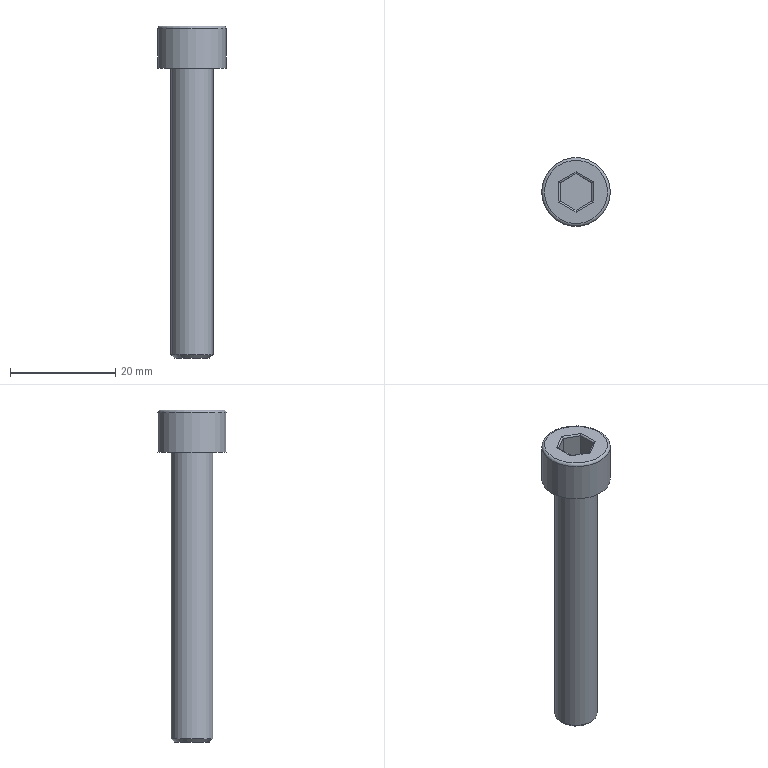Part | STEP file | 200 mesh_id90_xmt | 1 solid | 20 faces | box 13 x 13 x 63 mm | volume 3664 mm3 | plane 10 | cylinder 8 | torus 1 | cone 1 | commonest cylinder face diameters 0.6 x6 8 x1 13 x1
STEP:
#1=CARTESIAN_POINT('',(-16967.884,-4114.08,125.258));
#2=VERTEX_POINT('',#1);
#3=CARTESIAN_POINT('',(-16971.184,-4112.174,125.258));
#4=VERTEX_POINT('',#3);
#5=CARTESIAN_POINT('',(-16969.534,-4113.127,125.258));
#6=DIRECTION('',(-0.866,0.5,0.));
#7=VECTOR('',#6,1.);
#8=LINE('',#5,#7);
#9=EDGE_CURVE('',#2,#4,#8,.T.);
#10=ORIENTED_EDGE('',*,*,#9,.T.);
#11=CARTESIAN_POINT('',(-16971.184,-4108.364,125.258));
#12=VERTEX_POINT('',#11);
#13=CARTESIAN_POINT('',(-16971.184,-4110.269,125.258));
#14=DIRECTION('',(0.,1.,0.));
#15=VECTOR('',#14,1.);
#16=LINE('',#13,#15);
#17=EDGE_CURVE('',#4,#12,#16,.T.);
#18=ORIENTED_EDGE('',*,*,#17,.T.);
#19=CARTESIAN_POINT('',(-16967.884,-4106.459,125.258));
#20=VERTEX_POINT('',#19);
#21=CARTESIAN_POINT('',(-16969.534,-4107.411,125.258));
#22=DIRECTION('',(0.866,0.5,0.));
#23=VECTOR('',#22,1.);
#24=LINE('',#21,#23);
#25=EDGE_CURVE('',#12,#20,#24,.T.);
#26=ORIENTED_EDGE('',*,*,#25,.T.);
#27=CARTESIAN_POINT('',(-16964.584,-4108.364,125.258));
#28=VERTEX_POINT('',#27);
#29=CARTESIAN_POINT('',(-16966.234,-4107.411,125.258));
#30=DIRECTION('',(0.866,-0.5,0.));
#31=VECTOR('',#30,1.);
#32=LINE('',#29,#31);
#33=EDGE_CURVE('',#20,#28,#32,.T.);
#34=ORIENTED_EDGE('',*,*,#33,.T.);
#35=CARTESIAN_POINT('',(-16964.584,-4112.174,125.258));
#36=VERTEX_POINT('',#35);
#37=CARTESIAN_POINT('',(-16964.584,-4110.269,125.258));
#38=DIRECTION('',(0.,-1.,0.));
#39=VECTOR('',#38,1.);
#40=LINE('',#37,#39);
#41=EDGE_CURVE('',#28,#36,#40,.T.);
#42=ORIENTED_EDGE('',*,*,#41,.T.);
#43=CARTESIAN_POINT('',(-16966.234,-4113.127,125.258));
#44=DIRECTION('',(-0.866,-0.5,0.));
#45=VECTOR('',#44,1.);
#46=LINE('',#43,#45);
#47=EDGE_CURVE('',#36,#2,#46,.T.);
#48=ORIENTED_EDGE('',*,*,#47,.T.);
#49=EDGE_LOOP('',(#10,#18,#26,#34,#42,#48));
#50=FACE_BOUND('',#49,.T.);
#51=CARTESIAN_POINT('',(-16961.884,-4110.269,125.258));
#52=VERTEX_POINT('',#51);
#53=CARTESIAN_POINT('',(-16967.884,-4110.269,125.258));
#54=DIRECTION('',(0.,0.,1.));
#55=DIRECTION('',(1.,0.,0.));
#56=AXIS2_PLACEMENT_3D('',#53,#54,#55);
#57=CIRCLE('',#56,6.);
#58=EDGE_CURVE('',#52,#52,#57,.T.);
#59=ORIENTED_EDGE('',*,*,#58,.T.);
#60=EDGE_LOOP('',(#59));
#61=FACE_BOUND('',#60,.T.);
#62=CARTESIAN_POINT('',(-16967.884,-4110.269,125.258));
#63=DIRECTION('',(0.,0.,1.));
#64=DIRECTION('',(1.,0.,0.));
#65=AXIS2_PLACEMENT_3D('',#62,#63,#64);
#66=PLANE('',#65);
#67=ADVANCED_FACE('',(#50,#61),#66,.T.);
#68=CARTESIAN_POINT('',(-16971.884,-4110.269,62.858));
#69=VERTEX_POINT('',#68);
#70=CARTESIAN_POINT('',(-16967.884,-4110.269,62.858));
#71=DIRECTION('',(0.,0.,1.));
#72=DIRECTION('',(-1.,0.,0.));
#73=AXIS2_PLACEMENT_3D('',#70,#71,#72);
#74=CIRCLE('',#73,4.);
#75=EDGE_CURVE('',#69,#69,#74,.T.);
#76=ORIENTED_EDGE('',*,*,#75,.T.);
#77=EDGE_LOOP('',(#76));
#78=FACE_BOUND('',#77,.T.);
#79=CARTESIAN_POINT('',(-16971.884,-4110.269,117.258));
#80=VERTEX_POINT('',#79);
#81=CARTESIAN_POINT('',(-16967.884,-4110.269,117.258));
#82=DIRECTION('',(0.,0.,1.));
#83=DIRECTION('',(-1.,0.,0.));
#84=AXIS2_PLACEMENT_3D('',#81,#82,#83);
#85=CIRCLE('',#84,4.);
#86=EDGE_CURVE('',#80,#80,#85,.T.);
#87=ORIENTED_EDGE('',*,*,#86,.F.);
#88=EDGE_LOOP('',(#87));
#89=FACE_BOUND('',#88,.T.);
#90=CARTESIAN_POINT('',(-16967.884,-4110.269,117.258));
#91=DIRECTION('',(0.,0.,-1.));
#92=DIRECTION('',(1.,0.,0.));
#93=AXIS2_PLACEMENT_3D('',#90,#91,#92);
#94=CYLINDRICAL_SURFACE('',#93,4.);
#95=ADVANCED_FACE('',(#78,#89),#94,.T.);
#96=ORIENTED_EDGE('',*,*,#86,.T.);
#97=EDGE_LOOP('',(#96));
#98=FACE_BOUND('',#97,.T.);
#99=CARTESIAN_POINT('',(-16961.384,-4110.269,117.258));
#100=VERTEX_POINT('',#99);
#101=CARTESIAN_POINT('',(-16967.884,-4110.269,117.258));
#102=DIRECTION('',(0.,0.,1.));
#103=DIRECTION('',(1.,0.,0.));
#104=AXIS2_PLACEMENT_3D('',#101,#102,#103);
#105=CIRCLE('',#104,6.5);
#106=EDGE_CURVE('',#100,#100,#105,.T.);
#107=ORIENTED_EDGE('',*,*,#106,.F.);
#108=EDGE_LOOP('',(#107));
#109=FACE_BOUND('',#108,.T.);
#110=CARTESIAN_POINT('',(-16967.884,-4110.269,117.258));
#111=DIRECTION('',(0.,0.,-1.));
#112=DIRECTION('',(-1.,0.,0.));
#113=AXIS2_PLACEMENT_3D('',#110,#111,#112);
#114=PLANE('',#113);
#115=ADVANCED_FACE('',(#98,#109),#114,.T.);
#116=CARTESIAN_POINT('',(-16961.384,-4110.269,124.758));
#117=VERTEX_POINT('',#116);
#118=CARTESIAN_POINT('',(-16967.884,-4110.269,124.758));
#119=DIRECTION('',(0.,0.,-1.));
#120=DIRECTION('',(1.,0.,0.));
#121=AXIS2_PLACEMENT_3D('',#118,#119,#120);
#122=CIRCLE('',#121,6.5);
#123=EDGE_CURVE('',#117,#117,#122,.T.);
#124=ORIENTED_EDGE('',*,*,#123,.T.);
#125=EDGE_LOOP('',(#124));
#126=FACE_BOUND('',#125,.T.);
#127=ORIENTED_EDGE('',*,*,#106,.T.);
#128=EDGE_LOOP('',(#127));
#129=FACE_BOUND('',#128,.T.);
#130=CARTESIAN_POINT('',(-16967.884,-4110.269,117.258));
#131=DIRECTION('',(0.,0.,1.));
#132=DIRECTION('',(1.,0.,0.));
#133=AXIS2_PLACEMENT_3D('',#130,#131,#132);
#134=CYLINDRICAL_SURFACE('',#133,6.5);
#135=ADVANCED_FACE('',(#126,#129),#134,.T.);
#136=ORIENTED_EDGE('',*,*,#58,.F.);
#137=EDGE_LOOP('',(#136));
#138=FACE_BOUND('',#137,.T.);
#139=ORIENTED_EDGE('',*,*,#123,.F.);
#140=EDGE_LOOP('',(#139));
#141=FACE_BOUND('',#140,.T.);
#142=CARTESIAN_POINT('',(-16967.884,-4110.269,124.758));
#143=DIRECTION('',(0.,0.,1.));
#144=DIRECTION('',(1.,0.,0.));
#145=AXIS2_PLACEMENT_3D('',#142,#143,#144);
#146=TOROIDAL_SURFACE('',#145,6.,0.5);
#147=ADVANCED_FACE('',(#138,#141),#146,.T.);
#148=CARTESIAN_POINT('',(-16970.884,-4112.001,124.958));
#149=VERTEX_POINT('',#148);
#150=CARTESIAN_POINT('',(-16970.884,-4112.001,120.258));
#151=VERTEX_POINT('',#150);
#152=CARTESIAN_POINT('',(-16970.884,-4112.001,120.258));
#153=DIRECTION('',(0.,0.,-1.));
#154=VECTOR('',#153,1.);
#155=LINE('',#152,#154);
#156=EDGE_CURVE('',#149,#151,#155,.T.);
#157=ORIENTED_EDGE('',*,*,#156,.F.);
#158=CARTESIAN_POINT('',(-16967.884,-4113.733,124.958));
#159=VERTEX_POINT('',#158);
#160=CARTESIAN_POINT('',(-16967.884,-4113.733,124.958));
#161=DIRECTION('',(0.866,-0.5,0.));
#162=VECTOR('',#161,1.);
#163=LINE('',#160,#162);
#164=EDGE_CURVE('',#149,#159,#163,.T.);
#165=ORIENTED_EDGE('',*,*,#164,.T.);
#166=CARTESIAN_POINT('',(-16967.884,-4113.733,120.258));
#167=VERTEX_POINT('',#166);
#168=CARTESIAN_POINT('',(-16967.884,-4113.733,120.258));
#169=DIRECTION('',(0.,0.,-1.));
#170=VECTOR('',#169,1.);
#171=LINE('',#168,#170);
#172=EDGE_CURVE('',#159,#167,#171,.T.);
#173=ORIENTED_EDGE('',*,*,#172,.T.);
#174=CARTESIAN_POINT('',(-16967.884,-4113.733,120.258));
#175=DIRECTION('',(0.866,-0.5,0.));
#176=VECTOR('',#175,1.);
#177=LINE('',#174,#176);
#178=EDGE_CURVE('',#151,#167,#177,.T.);
#179=ORIENTED_EDGE('',*,*,#178,.F.);
#180=EDGE_LOOP('',(#157,#165,#173,#179));
#181=FACE_OUTER_BOUND('',#180,.T.);
#182=CARTESIAN_POINT('',(-16967.884,-4113.733,120.258));
#183=DIRECTION('',(0.5,0.866,0.));
#184=DIRECTION('',(-0.866,0.5,0.));
#185=AXIS2_PLACEMENT_3D('',#182,#183,#184);
#186=PLANE('',#185);
#187=ADVANCED_FACE('',(#181),#186,.T.);
#188=CARTESIAN_POINT('',(-16970.884,-4108.537,124.958));
#189=VERTEX_POINT('',#188);
#190=CARTESIAN_POINT('',(-16970.884,-4108.537,120.258));
#191=VERTEX_POINT('',#190);
#192=CARTESIAN_POINT('',(-16970.884,-4108.537,120.258));
#193=DIRECTION('',(0.,0.,-1.));
#194=VECTOR('',#193,1.);
#195=LINE('',#192,#194);
#196=EDGE_CURVE('',#189,#191,#195,.T.);
#197=ORIENTED_EDGE('',*,*,#196,.F.);
#198=CARTESIAN_POINT('',(-16970.884,-4112.001,124.958));
#199=DIRECTION('',(0.,-1.,0.));
#200=VECTOR('',#199,1.);
#201=LINE('',#198,#200);
#202=EDGE_CURVE('',#189,#149,#201,.T.);
#203=ORIENTED_EDGE('',*,*,#202,.T.);
#204=ORIENTED_EDGE('',*,*,#156,.T.);
#205=CARTESIAN_POINT('',(-16970.884,-4112.001,120.258));
#206=DIRECTION('',(0.,-1.,0.));
#207=VECTOR('',#206,1.);
#208=LINE('',#205,#207);
#209=EDGE_CURVE('',#191,#151,#208,.T.);
#210=ORIENTED_EDGE('',*,*,#209,.F.);
#211=EDGE_LOOP('',(#197,#203,#204,#210));
#212=FACE_OUTER_BOUND('',#211,.T.);
#213=CARTESIAN_POINT('',(-16970.884,-4112.001,120.258));
#214=DIRECTION('',(1.,0.,0.));
#215=DIRECTION('',(0.,0.,-1.));
#216=AXIS2_PLACEMENT_3D('',#213,#214,#215);
#217=PLANE('',#216);
#218=ADVANCED_FACE('',(#212),#217,.T.);
#219=CARTESIAN_POINT('',(-16967.884,-4106.805,124.958));
#220=VERTEX_POINT('',#219);
#221=CARTESIAN_POINT('',(-16967.884,-4106.805,120.258));
#222=VERTEX_POINT('',#221);
#223=CARTESIAN_POINT('',(-16967.884,-4106.805,120.258));
#224=DIRECTION('',(0.,0.,-1.));
#225=VECTOR('',#224,1.);
#226=LINE('',#223,#225);
#227=EDGE_CURVE('',#220,#222,#226,.T.);
#228=ORIENTED_EDGE('',*,*,#227,.F.);
#229=CARTESIAN_POINT('',(-16970.884,-4108.537,124.958));
#230=DIRECTION('',(-0.866,-0.5,0.));
#231=VECTOR('',#230,1.);
#232=LINE('',#229,#231);
#233=EDGE_CURVE('',#220,#189,#232,.T.);
#234=ORIENTED_EDGE('',*,*,#233,.T.);
#235=ORIENTED_EDGE('',*,*,#196,.T.);
#236=CARTESIAN_POINT('',(-16970.884,-4108.537,120.258));
#237=DIRECTION('',(-0.866,-0.5,0.));
#238=VECTOR('',#237,1.);
#239=LINE('',#236,#238);
#240=EDGE_CURVE('',#222,#191,#239,.T.);
#241=ORIENTED_EDGE('',*,*,#240,.F.);
#242=EDGE_LOOP('',(#228,#234,#235,#241));
#243=FACE_OUTER_BOUND('',#242,.T.);
#244=CARTESIAN_POINT('',(-16970.884,-4108.537,120.258));
#245=DIRECTION('',(0.5,-0.866,0.));
#246=DIRECTION('',(0.866,0.5,0.));
#247=AXIS2_PLACEMENT_3D('',#244,#245,#246);
#248=PLANE('',#247);
#249=ADVANCED_FACE('',(#243),#248,.T.);
#250=CARTESIAN_POINT('',(-16964.884,-4108.537,124.958));
#251=VERTEX_POINT('',#250);
#252=CARTESIAN_POINT('',(-16964.884,-4108.537,120.258));
#253=VERTEX_POINT('',#252);
#254=CARTESIAN_POINT('',(-16964.884,-4108.537,120.258));
#255=DIRECTION('',(0.,0.,-1.));
#256=VECTOR('',#255,1.);
#257=LINE('',#254,#256);
#258=EDGE_CURVE('',#251,#253,#257,.T.);
#259=ORIENTED_EDGE('',*,*,#258,.F.);
#260=CARTESIAN_POINT('',(-16967.884,-4106.805,124.958));
#261=DIRECTION('',(-0.866,0.5,0.));
#262=VECTOR('',#261,1.);
#263=LINE('',#260,#262);
#264=EDGE_CURVE('',#251,#220,#263,.T.);
#265=ORIENTED_EDGE('',*,*,#264,.T.);
#266=ORIENTED_EDGE('',*,*,#227,.T.);
#267=CARTESIAN_POINT('',(-16967.884,-4106.805,120.258));
#268=DIRECTION('',(-0.866,0.5,0.));
#269=VECTOR('',#268,1.);
#270=LINE('',#267,#269);
#271=EDGE_CURVE('',#253,#222,#270,.T.);
#272=ORIENTED_EDGE('',*,*,#271,.F.);
#273=EDGE_LOOP('',(#259,#265,#266,#272));
#274=FACE_OUTER_BOUND('',#273,.T.);
#275=CARTESIAN_POINT('',(-16967.884,-4106.805,120.258));
#276=DIRECTION('',(-0.5,-0.866,0.));
#277=DIRECTION('',(0.866,-0.5,0.));
#278=AXIS2_PLACEMENT_3D('',#275,#276,#277);
#279=PLANE('',#278);
#280=ADVANCED_FACE('',(#274),#279,.T.);
#281=CARTESIAN_POINT('',(-16964.884,-4112.001,124.958));
#282=VERTEX_POINT('',#281);
#283=CARTESIAN_POINT('',(-16964.884,-4112.001,120.258));
#284=VERTEX_POINT('',#283);
#285=CARTESIAN_POINT('',(-16964.884,-4112.001,120.258));
#286=DIRECTION('',(0.,0.,-1.));
#287=VECTOR('',#286,1.);
#288=LINE('',#285,#287);
#289=EDGE_CURVE('',#282,#284,#288,.T.);
#290=ORIENTED_EDGE('',*,*,#289,.F.);
#291=CARTESIAN_POINT('',(-16964.884,-4108.537,124.958));
#292=DIRECTION('',(0.,1.,0.));
#293=VECTOR('',#292,1.);
#294=LINE('',#291,#293);
#295=EDGE_CURVE('',#282,#251,#294,.T.);
#296=ORIENTED_EDGE('',*,*,#295,.T.);
#297=ORIENTED_EDGE('',*,*,#258,.T.);
#298=CARTESIAN_POINT('',(-16964.884,-4108.537,120.258));
#299=DIRECTION('',(0.,1.,0.));
#300=VECTOR('',#299,1.);
#301=LINE('',#298,#300);
#302=EDGE_CURVE('',#284,#253,#301,.T.);
#303=ORIENTED_EDGE('',*,*,#302,.F.);
#304=EDGE_LOOP('',(#290,#296,#297,#303));
#305=FACE_OUTER_BOUND('',#304,.T.);
#306=CARTESIAN_POINT('',(-16964.884,-4108.537,120.258));
#307=DIRECTION('',(-1.,0.,0.));
#308=DIRECTION('',(0.,0.,1.));
#309=AXIS2_PLACEMENT_3D('',#306,#307,#308);
#310=PLANE('',#309);
#311=ADVANCED_FACE('',(#305),#310,.T.);
#312=ORIENTED_EDGE('',*,*,#172,.F.);
#313=CARTESIAN_POINT('',(-16964.884,-4112.001,124.958));
#314=DIRECTION('',(0.866,0.5,0.));
#315=VECTOR('',#314,1.);
#316=LINE('',#313,#315);
#317=EDGE_CURVE('',#159,#282,#316,.T.);
#318=ORIENTED_EDGE('',*,*,#317,.T.);
#319=ORIENTED_EDGE('',*,*,#289,.T.);
#320=CARTESIAN_POINT('',(-16964.884,-4112.001,120.258));
#321=DIRECTION('',(0.866,0.5,0.));
#322=VECTOR('',#321,1.);
#323=LINE('',#320,#322);
#324=EDGE_CURVE('',#167,#284,#323,.T.);
#325=ORIENTED_EDGE('',*,*,#324,.F.);
#326=EDGE_LOOP('',(#312,#318,#319,#325));
#327=FACE_OUTER_BOUND('',#326,.T.);
#328=CARTESIAN_POINT('',(-16964.884,-4112.001,120.258));
#329=DIRECTION('',(-0.5,0.866,0.));
#330=DIRECTION('',(-0.866,-0.5,0.));
#331=AXIS2_PLACEMENT_3D('',#328,#329,#330);
#332=PLANE('',#331);
#333=ADVANCED_FACE('',(#327),#332,.T.);
#334=ORIENTED_EDGE('',*,*,#178,.T.);
#335=ORIENTED_EDGE('',*,*,#324,.T.);
#336=ORIENTED_EDGE('',*,*,#302,.T.);
#337=ORIENTED_EDGE('',*,*,#271,.T.);
#338=ORIENTED_EDGE('',*,*,#240,.T.);
#339=ORIENTED_EDGE('',*,*,#209,.T.);
#340=EDGE_LOOP('',(#334,#335,#336,#337,#338,#339));
#341=FACE_OUTER_BOUND('',#340,.T.);
#342=CARTESIAN_POINT('',(0.,-175.,120.258));
#343=DIRECTION('',(0.,0.,-1.));
#344=DIRECTION('',(-1.,0.,0.));
#345=AXIS2_PLACEMENT_3D('',#342,#343,#344);
#346=PLANE('',#345);
#347=ADVANCED_FACE('',(#341),#346,.F.);
#348=CARTESIAN_POINT('',(-16964.584,-4108.364,124.958));
#349=DIRECTION('',(-0.5,0.866,0.));
#350=DIRECTION('',(0.866,0.5,0.));
#351=AXIS2_PLACEMENT_3D('',#348,#349,#350);
#352=ELLIPSE('',#351,0.3464,0.3);
#353=EDGE_CURVE('',#251,#28,#352,.T.);
#354=ORIENTED_EDGE('',*,*,#353,.F.);
#355=ORIENTED_EDGE('',*,*,#295,.F.);
#356=CARTESIAN_POINT('',(-16964.584,-4112.174,124.958));
#357=DIRECTION('',(-0.5,-0.866,0.));
#358=DIRECTION('',(0.866,-0.5,0.));
#359=AXIS2_PLACEMENT_3D('',#356,#357,#358);
#360=ELLIPSE('',#359,0.3464,0.3);
#361=EDGE_CURVE('',#36,#282,#360,.T.);
#362=ORIENTED_EDGE('',*,*,#361,.F.);
#363=ORIENTED_EDGE('',*,*,#41,.F.);
#364=EDGE_LOOP('',(#354,#355,#362,#363));
#365=FACE_OUTER_BOUND('',#364,.T.);
#366=CARTESIAN_POINT('',(-16964.584,-4110.269,124.958));
#367=DIRECTION('',(0.,-1.,0.));
#368=DIRECTION('',(0.,0.,-1.));
#369=AXIS2_PLACEMENT_3D('',#366,#367,#368);
#370=CYLINDRICAL_SURFACE('',#369,0.3);
#371=ADVANCED_FACE('',(#365),#370,.T.);
#372=ORIENTED_EDGE('',*,*,#361,.T.);
#373=ORIENTED_EDGE('',*,*,#317,.F.);
#374=CARTESIAN_POINT('',(-16967.884,-4114.08,124.958));
#375=DIRECTION('',(-1.,0.,0.));
#376=DIRECTION('',(0.,-1.,0.));
#377=AXIS2_PLACEMENT_3D('',#374,#375,#376);
#378=ELLIPSE('',#377,0.3464,0.3);
#379=EDGE_CURVE('',#2,#159,#378,.T.);
#380=ORIENTED_EDGE('',*,*,#379,.F.);
#381=ORIENTED_EDGE('',*,*,#47,.F.);
#382=EDGE_LOOP('',(#372,#373,#380,#381));
#383=FACE_OUTER_BOUND('',#382,.T.);
#384=CARTESIAN_POINT('',(-16966.234,-4113.127,124.958));
#385=DIRECTION('',(-0.866,-0.5,0.));
#386=DIRECTION('',(0.5,-0.866,0.));
#387=AXIS2_PLACEMENT_3D('',#384,#385,#386);
#388=CYLINDRICAL_SURFACE('',#387,0.3);
#389=ADVANCED_FACE('',(#383),#388,.T.);
#390=ORIENTED_EDGE('',*,*,#353,.T.);
#391=ORIENTED_EDGE('',*,*,#33,.F.);
#392=CARTESIAN_POINT('',(-16967.884,-4106.459,124.958));
#393=DIRECTION('',(-1.,0.,0.));
#394=DIRECTION('',(0.,1.,0.));
#395=AXIS2_PLACEMENT_3D('',#392,#393,#394);
#396=ELLIPSE('',#395,0.3464,0.3);
#397=EDGE_CURVE('',#220,#20,#396,.T.);
#398=ORIENTED_EDGE('',*,*,#397,.F.);
#399=ORIENTED_EDGE('',*,*,#264,.F.);
#400=EDGE_LOOP('',(#390,#391,#398,#399));
#401=FACE_OUTER_BOUND('',#400,.T.);
#402=CARTESIAN_POINT('',(-16966.234,-4107.411,124.958));
#403=DIRECTION('',(0.866,-0.5,0.));
#404=DIRECTION('',(0.5,0.866,0.));
#405=AXIS2_PLACEMENT_3D('',#402,#403,#404);
#406=CYLINDRICAL_SURFACE('',#405,0.3);
#407=ADVANCED_FACE('',(#401),#406,.T.);
#408=ORIENTED_EDGE('',*,*,#379,.T.);
#409=ORIENTED_EDGE('',*,*,#164,.F.);
#410=CARTESIAN_POINT('',(-16971.184,-4112.174,124.958));
#411=DIRECTION('',(-0.5,0.866,0.));
#412=DIRECTION('',(0.866,0.5,0.));
#413=AXIS2_PLACEMENT_3D('',#410,#411,#412);
#414=ELLIPSE('',#413,0.3464,0.3);
#415=EDGE_CURVE('',#4,#149,#414,.T.);
#416=ORIENTED_EDGE('',*,*,#415,.F.);
#417=ORIENTED_EDGE('',*,*,#9,.F.);
#418=EDGE_LOOP('',(#408,#409,#416,#417));
#419=FACE_OUTER_BOUND('',#418,.T.);
#420=CARTESIAN_POINT('',(-16969.534,-4113.127,124.958));
#421=DIRECTION('',(-0.866,0.5,0.));
#422=DIRECTION('',(-0.5,-0.866,0.));
#423=AXIS2_PLACEMENT_3D('',#420,#421,#422);
#424=CYLINDRICAL_SURFACE('',#423,0.3);
#425=ADVANCED_FACE('',(#419),#424,.T.);
#426=ORIENTED_EDGE('',*,*,#397,.T.);
#427=ORIENTED_EDGE('',*,*,#25,.F.);
#428=CARTESIAN_POINT('',(-16971.184,-4108.364,124.958));
#429=DIRECTION('',(-0.5,-0.866,0.));
#430=DIRECTION('',(-0.866,0.5,0.));
#431=AXIS2_PLACEMENT_3D('',#428,#429,#430);
#432=ELLIPSE('',#431,0.3464,0.3);
#433=EDGE_CURVE('',#189,#12,#432,.T.);
#434=ORIENTED_EDGE('',*,*,#433,.F.);
#435=ORIENTED_EDGE('',*,*,#233,.F.);
#436=EDGE_LOOP('',(#426,#427,#434,#435));
#437=FACE_OUTER_BOUND('',#436,.T.);
#438=CARTESIAN_POINT('',(-16969.534,-4107.411,124.958));
#439=DIRECTION('',(0.866,0.5,0.));
#440=DIRECTION('',(-0.5,0.866,0.));
#441=AXIS2_PLACEMENT_3D('',#438,#439,#440);
#442=CYLINDRICAL_SURFACE('',#441,0.3);
#443=ADVANCED_FACE('',(#437),#442,.T.);
#444=ORIENTED_EDGE('',*,*,#415,.T.);
#445=ORIENTED_EDGE('',*,*,#202,.F.);
#446=ORIENTED_EDGE('',*,*,#433,.T.);
#447=ORIENTED_EDGE('',*,*,#17,.F.);
#448=EDGE_LOOP('',(#444,#445,#446,#447));
#449=FACE_OUTER_BOUND('',#448,.T.);
#450=CARTESIAN_POINT('',(-16971.184,-4110.269,124.958));
#451=DIRECTION('',(0.,1.,0.));
#452=DIRECTION('',(0.,0.,1.));
#453=AXIS2_PLACEMENT_3D('',#450,#451,#452);
#454=CYLINDRICAL_SURFACE('',#453,0.3);
#455=ADVANCED_FACE('',(#449),#454,.T.);
#456=CARTESIAN_POINT('',(-16971.284,-4110.269,62.258));
#457=VERTEX_POINT('',#456);
#458=CARTESIAN_POINT('',(-16967.884,-4110.269,62.258));
#459=DIRECTION('',(0.,0.,-1.));
#460=DIRECTION('',(-1.,0.,0.));
#461=AXIS2_PLACEMENT_3D('',#458,#459,#460);
#462=CIRCLE('',#461,3.4);
#463=EDGE_CURVE('',#457,#457,#462,.T.);
#464=ORIENTED_EDGE('',*,*,#463,.T.);
#465=EDGE_LOOP('',(#464));
#466=FACE_OUTER_BOUND('',#465,.T.);
#467=CARTESIAN_POINT('',(-16967.884,-4110.269,62.258));
#468=DIRECTION('',(0.,0.,-1.));
#469=DIRECTION('',(-1.,0.,0.));
#470=AXIS2_PLACEMENT_3D('',#467,#468,#469);
#471=PLANE('',#470);
#472=ADVANCED_FACE('',(#466),#471,.T.);
#473=ORIENTED_EDGE('',*,*,#463,.F.);
#474=EDGE_LOOP('',(#473));
#475=FACE_BOUND('',#474,.T.);
#476=ORIENTED_EDGE('',*,*,#75,.F.);
#477=EDGE_LOOP('',(#476));
#478=FACE_BOUND('',#477,.T.);
#479=CARTESIAN_POINT('',(-16967.884,-4110.269,62.858));
#480=DIRECTION('',(0.,0.,1.));
#481=DIRECTION('',(1.,0.,0.));
#482=AXIS2_PLACEMENT_3D('',#479,#480,#481);
#483=CONICAL_SURFACE('',#482,4.,45.);
#484=ADVANCED_FACE('',(#475,#478),#483,.T.);
#485=CLOSED_SHELL('',(#67,#95,#115,#135,#147,#187,#218,#249,#280,#311,#333,#347,#371,#389,#407,#425,#443,#455,#472,#484));
#486=MANIFOLD_SOLID_BREP('',#485);
#487=(LENGTH_UNIT()NAMED_UNIT(*)SI_UNIT(.MILLI.,.METRE.));
#488=UNCERTAINTY_MEASURE_WITH_UNIT(LENGTH_MEASURE(0.00002),#487,'','');
#489=(NAMED_UNIT(*)PLANE_ANGLE_UNIT()SI_UNIT($,.RADIAN.));
#490=PLANE_ANGLE_MEASURE_WITH_UNIT(PLANE_ANGLE_MEASURE(0.01745),#489);
#491=DIMENSIONAL_EXPONENTS(0.,0.,0.,0.,0.,0.,0.);
#492=(CONVERSION_BASED_UNIT('DEGREE',#490)NAMED_UNIT(#491)PLANE_ANGLE_UNIT());
#493=(NAMED_UNIT(*)SI_UNIT($,.STERADIAN.)SOLID_ANGLE_UNIT());
#494=(GEOMETRIC_REPRESENTATION_CONTEXT(3)GLOBAL_UNCERTAINTY_ASSIGNED_CONTEXT((#488))GLOBAL_UNIT_ASSIGNED_CONTEXT((#487,#492,#493))REPRESENTATION_CONTEXT('',''));
#495=ADVANCED_BREP_SHAPE_REPRESENTATION('',(#486),#494);